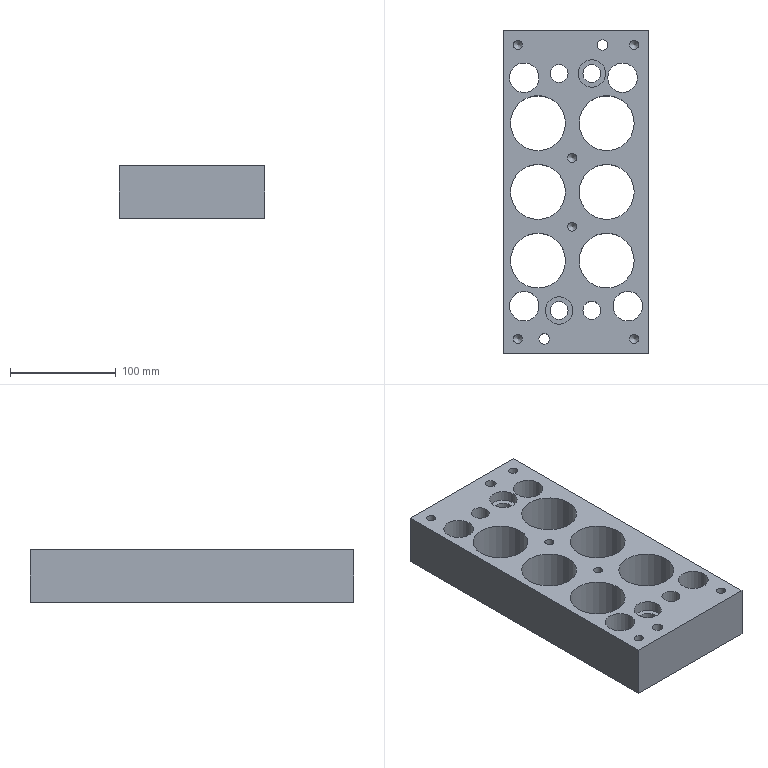Part | NX | features solid 2 | 1 solid | 82 faces | box 138 x 306 x 50 mm | volume 1260967 mm3 | cylinder 46 | plane 22 | cone 14 | commonest cylinder face diameters 5.199 x8 11 x8 8.499 x6 52 x6 17 x4 28 x4